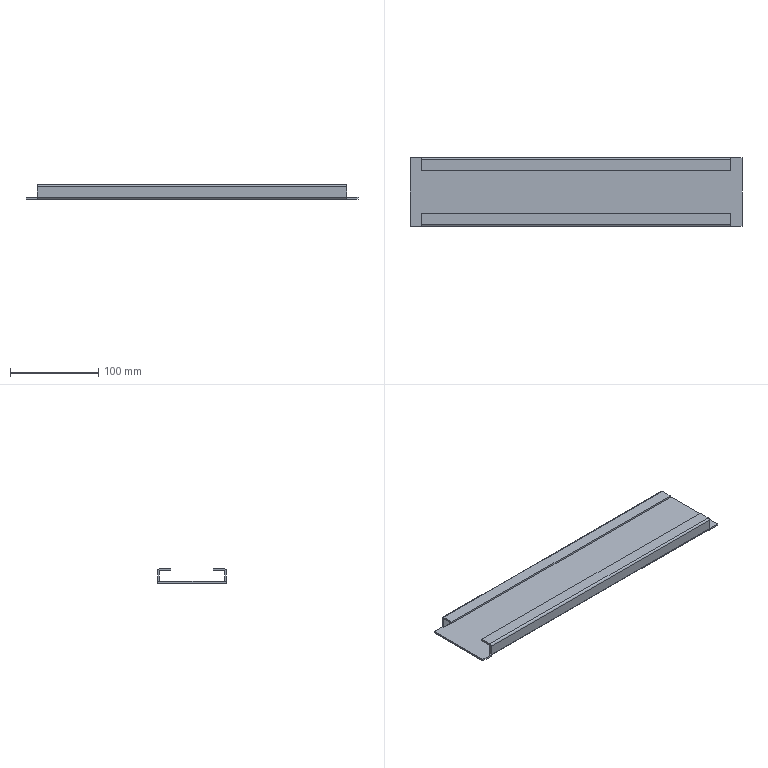Part | STEP file | SX-022-03 | 1 solid | 46 faces | box 376 x 78 x 16 mm | volume 95014 mm3 | plane 38 | cylinder 8 | commonest cylinder face diameters 0.4 x4 4.4 x4